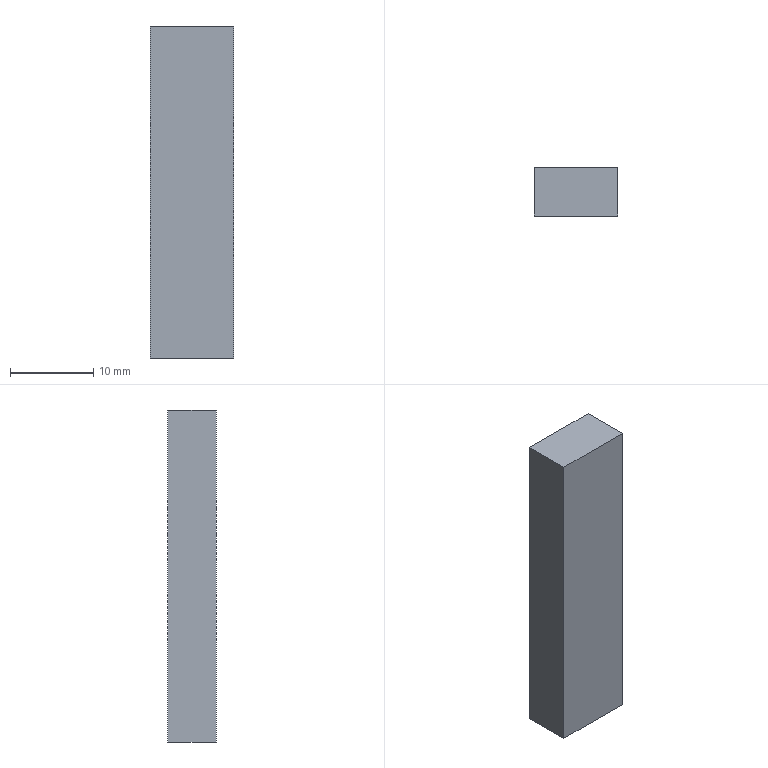Part | NX | features solid 2 | 1 solid | 6 faces | box 10 x 5.859 x 40 mm | volume 2343 mm3 | plane 6
STEP:
#1=CARTESIAN_POINT('',(2250.,-204.541,260.));
#2=VERTEX_POINT('',#1);
#3=CARTESIAN_POINT('',(2250.,-210.4,260.));
#4=VERTEX_POINT('',#3);
#5=CARTESIAN_POINT('',(2250.,-204.541,260.));
#6=CARTESIAN_POINT('',(2250.,-206.494,260.));
#7=CARTESIAN_POINT('',(2250.,-208.447,260.));
#8=CARTESIAN_POINT('',(2250.,-210.4,260.));
#9=B_SPLINE_CURVE_WITH_KNOTS('',3,(#5,#6,#7,#8),.UNSPECIFIED.,.F.,.F.,(4,4),(0.,0.06388),.PIECEWISE_BEZIER_KNOTS.);
#10=EDGE_CURVE('',#2,#4,#9,.T.);
#11=ORIENTED_EDGE('',*,*,#10,.F.);
#12=CARTESIAN_POINT('',(2260.,-204.541,260.));
#13=VERTEX_POINT('',#12);
#14=CARTESIAN_POINT('',(2260.,-204.541,260.));
#15=DIRECTION('',(-1.,0.,0.));
#16=VECTOR('',#15,1000.);
#17=LINE('',#14,#16);
#18=EDGE_CURVE('',#13,#2,#17,.T.);
#19=ORIENTED_EDGE('',*,*,#18,.F.);
#20=CARTESIAN_POINT('',(2260.,-210.4,260.));
#21=VERTEX_POINT('',#20);
#22=CARTESIAN_POINT('',(2260.,-204.541,260.));
#23=CARTESIAN_POINT('',(2260.,-206.494,260.));
#24=CARTESIAN_POINT('',(2260.,-208.447,260.));
#25=CARTESIAN_POINT('',(2260.,-210.4,260.));
#26=B_SPLINE_CURVE_WITH_KNOTS('',3,(#22,#23,#24,#25),.UNSPECIFIED.,.F.,.F.,(4,4),(0.,0.06388),.PIECEWISE_BEZIER_KNOTS.);
#27=EDGE_CURVE('',#13,#21,#26,.T.);
#28=ORIENTED_EDGE('',*,*,#27,.T.);
#29=CARTESIAN_POINT('',(2260.,-210.4,260.));
#30=DIRECTION('',(-1.,0.,0.));
#31=VECTOR('',#30,1000.);
#32=LINE('',#29,#31);
#33=EDGE_CURVE('',#21,#4,#32,.T.);
#34=ORIENTED_EDGE('',*,*,#33,.T.);
#35=EDGE_LOOP('',(#11,#19,#28,#34));
#36=FACE_BOUND('',#35,.T.);
#37=CARTESIAN_POINT('',(2260.,-204.541,260.));
#38=DIRECTION('',(0.,0.,-1.));
#39=DIRECTION('',(-1.,0.,0.));
#40=AXIS2_PLACEMENT_3D('',#37,#38,#39);
#41=PLANE('',#40);
#42=ADVANCED_FACE('',(#36),#41,.T.);
#43=CARTESIAN_POINT('',(2250.,-210.4,300.));
#44=VERTEX_POINT('',#43);
#45=CARTESIAN_POINT('',(2250.,-210.4,260.));
#46=CARTESIAN_POINT('',(2250.,-210.4,273.333));
#47=CARTESIAN_POINT('',(2250.,-210.4,286.667));
#48=CARTESIAN_POINT('',(2250.,-210.4,300.));
#49=B_SPLINE_CURVE_WITH_KNOTS('',3,(#45,#46,#47,#48),.UNSPECIFIED.,.F.,.F.,(4,4),(0.06388,0.5),.PIECEWISE_BEZIER_KNOTS.);
#50=EDGE_CURVE('',#4,#44,#49,.T.);
#51=ORIENTED_EDGE('',*,*,#50,.F.);
#52=ORIENTED_EDGE('',*,*,#33,.F.);
#53=CARTESIAN_POINT('',(2260.,-210.4,300.));
#54=VERTEX_POINT('',#53);
#55=CARTESIAN_POINT('',(2260.,-210.4,260.));
#56=CARTESIAN_POINT('',(2260.,-210.4,273.333));
#57=CARTESIAN_POINT('',(2260.,-210.4,286.667));
#58=CARTESIAN_POINT('',(2260.,-210.4,300.));
#59=B_SPLINE_CURVE_WITH_KNOTS('',3,(#55,#56,#57,#58),.UNSPECIFIED.,.F.,.F.,(4,4),(0.06388,0.5),.PIECEWISE_BEZIER_KNOTS.);
#60=EDGE_CURVE('',#21,#54,#59,.T.);
#61=ORIENTED_EDGE('',*,*,#60,.T.);
#62=CARTESIAN_POINT('',(2260.,-210.4,300.));
#63=DIRECTION('',(-1.,0.,0.));
#64=VECTOR('',#63,1000.);
#65=LINE('',#62,#64);
#66=EDGE_CURVE('',#54,#44,#65,.T.);
#67=ORIENTED_EDGE('',*,*,#66,.T.);
#68=EDGE_LOOP('',(#51,#52,#61,#67));
#69=FACE_BOUND('',#68,.T.);
#70=CARTESIAN_POINT('',(2260.,-210.4,260.));
#71=DIRECTION('',(0.,-1.,0.));
#72=DIRECTION('',(1.,0.,0.));
#73=AXIS2_PLACEMENT_3D('',#70,#71,#72);
#74=PLANE('',#73);
#75=ADVANCED_FACE('',(#69),#74,.T.);
#76=CARTESIAN_POINT('',(2250.,-204.541,300.));
#77=VERTEX_POINT('',#76);
#78=CARTESIAN_POINT('',(2250.,-210.4,300.));
#79=CARTESIAN_POINT('',(2250.,-208.447,300.));
#80=CARTESIAN_POINT('',(2250.,-206.494,300.));
#81=CARTESIAN_POINT('',(2250.,-204.541,300.));
#82=B_SPLINE_CURVE_WITH_KNOTS('',3,(#78,#79,#80,#81),.UNSPECIFIED.,.F.,.F.,(4,4),(0.5,0.5639),.PIECEWISE_BEZIER_KNOTS.);
#83=EDGE_CURVE('',#44,#77,#82,.T.);
#84=ORIENTED_EDGE('',*,*,#83,.F.);
#85=ORIENTED_EDGE('',*,*,#66,.F.);
#86=CARTESIAN_POINT('',(2260.,-204.541,300.));
#87=VERTEX_POINT('',#86);
#88=CARTESIAN_POINT('',(2260.,-210.4,300.));
#89=CARTESIAN_POINT('',(2260.,-208.447,300.));
#90=CARTESIAN_POINT('',(2260.,-206.494,300.));
#91=CARTESIAN_POINT('',(2260.,-204.541,300.));
#92=B_SPLINE_CURVE_WITH_KNOTS('',3,(#88,#89,#90,#91),.UNSPECIFIED.,.F.,.F.,(4,4),(0.5,0.5639),.PIECEWISE_BEZIER_KNOTS.);
#93=EDGE_CURVE('',#54,#87,#92,.T.);
#94=ORIENTED_EDGE('',*,*,#93,.T.);
#95=CARTESIAN_POINT('',(2260.,-204.541,300.));
#96=DIRECTION('',(-1.,0.,0.));
#97=VECTOR('',#96,1000.);
#98=LINE('',#95,#97);
#99=EDGE_CURVE('',#87,#77,#98,.T.);
#100=ORIENTED_EDGE('',*,*,#99,.T.);
#101=EDGE_LOOP('',(#84,#85,#94,#100));
#102=FACE_BOUND('',#101,.T.);
#103=CARTESIAN_POINT('',(2260.,-210.4,300.));
#104=DIRECTION('',(0.,0.,1.));
#105=DIRECTION('',(1.,0.,0.));
#106=AXIS2_PLACEMENT_3D('',#103,#104,#105);
#107=PLANE('',#106);
#108=ADVANCED_FACE('',(#102),#107,.T.);
#109=CARTESIAN_POINT('',(2250.,-204.541,300.));
#110=CARTESIAN_POINT('',(2250.,-204.541,286.667));
#111=CARTESIAN_POINT('',(2250.,-204.541,273.333));
#112=CARTESIAN_POINT('',(2250.,-204.541,260.));
#113=B_SPLINE_CURVE_WITH_KNOTS('',3,(#109,#110,#111,#112),.UNSPECIFIED.,.F.,.F.,(4,4),(0.5639,1.),.PIECEWISE_BEZIER_KNOTS.);
#114=EDGE_CURVE('',#77,#2,#113,.T.);
#115=ORIENTED_EDGE('',*,*,#114,.F.);
#116=ORIENTED_EDGE('',*,*,#99,.F.);
#117=CARTESIAN_POINT('',(2260.,-204.541,300.));
#118=CARTESIAN_POINT('',(2260.,-204.541,286.667));
#119=CARTESIAN_POINT('',(2260.,-204.541,273.333));
#120=CARTESIAN_POINT('',(2260.,-204.541,260.));
#121=B_SPLINE_CURVE_WITH_KNOTS('',3,(#117,#118,#119,#120),.UNSPECIFIED.,.F.,.F.,(4,4),(0.5639,1.),.PIECEWISE_BEZIER_KNOTS.);
#122=EDGE_CURVE('',#87,#13,#121,.T.);
#123=ORIENTED_EDGE('',*,*,#122,.T.);
#124=ORIENTED_EDGE('',*,*,#18,.T.);
#125=EDGE_LOOP('',(#115,#116,#123,#124));
#126=FACE_BOUND('',#125,.T.);
#127=CARTESIAN_POINT('',(2260.,-204.541,300.));
#128=DIRECTION('',(0.,1.,0.));
#129=DIRECTION('',(-1.,0.,0.));
#130=AXIS2_PLACEMENT_3D('',#127,#128,#129);
#131=PLANE('',#130);
#132=ADVANCED_FACE('',(#126),#131,.T.);
#133=ORIENTED_EDGE('',*,*,#27,.F.);
#134=ORIENTED_EDGE('',*,*,#122,.F.);
#135=ORIENTED_EDGE('',*,*,#93,.F.);
#136=ORIENTED_EDGE('',*,*,#60,.F.);
#137=EDGE_LOOP('',(#133,#134,#135,#136));
#138=FACE_BOUND('',#137,.T.);
#139=CARTESIAN_POINT('',(2260.,-207.471,260.));
#140=DIRECTION('',(1.,0.,0.));
#141=DIRECTION('',(0.,1.,0.));
#142=AXIS2_PLACEMENT_3D('',#139,#140,#141);
#143=PLANE('',#142);
#144=ADVANCED_FACE('',(#138),#143,.T.);
#145=ORIENTED_EDGE('',*,*,#10,.T.);
#146=ORIENTED_EDGE('',*,*,#50,.T.);
#147=ORIENTED_EDGE('',*,*,#83,.T.);
#148=ORIENTED_EDGE('',*,*,#114,.T.);
#149=EDGE_LOOP('',(#145,#146,#147,#148));
#150=FACE_BOUND('',#149,.T.);
#151=CARTESIAN_POINT('',(2250.,-207.471,260.));
#152=DIRECTION('',(1.,0.,0.));
#153=DIRECTION('',(0.,1.,0.));
#154=AXIS2_PLACEMENT_3D('',#151,#152,#153);
#155=PLANE('',#154);
#156=ADVANCED_FACE('',(#150),#155,.F.);
#157=CLOSED_SHELL('',(#42,#75,#108,#132,#144,#156));
#158=MANIFOLD_SOLID_BREP('',#157);
#159=(LENGTH_UNIT()NAMED_UNIT(*)SI_UNIT(.MILLI.,.METRE.));
#160=UNCERTAINTY_MEASURE_WITH_UNIT(LENGTH_MEASURE(0.00001),#159,'','');
#161=(NAMED_UNIT(*)PLANE_ANGLE_UNIT()SI_UNIT($,.RADIAN.));
#162=(NAMED_UNIT(*)SI_UNIT($,.STERADIAN.)SOLID_ANGLE_UNIT());
#163=(GEOMETRIC_REPRESENTATION_CONTEXT(3)GLOBAL_UNCERTAINTY_ASSIGNED_CONTEXT((#160))GLOBAL_UNIT_ASSIGNED_CONTEXT((#159,#161,#162))REPRESENTATION_CONTEXT('',''));
#164=ADVANCED_BREP_SHAPE_REPRESENTATION('',(#158),#163);